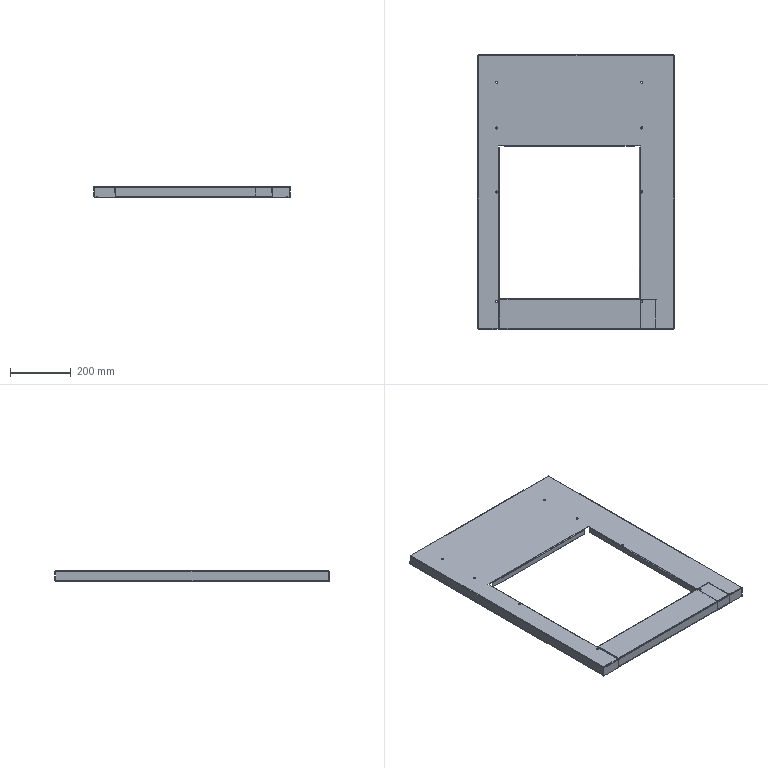Part | SolidWorks | 2 solids | 200 faces | box 645 x 900 x 35 mm | volume 1036306 mm3 | plane 110 | cylinder 78 | spline 12 | commonest cylinder face diameters 6.8 x30 2 x16 6 x16 7 x16